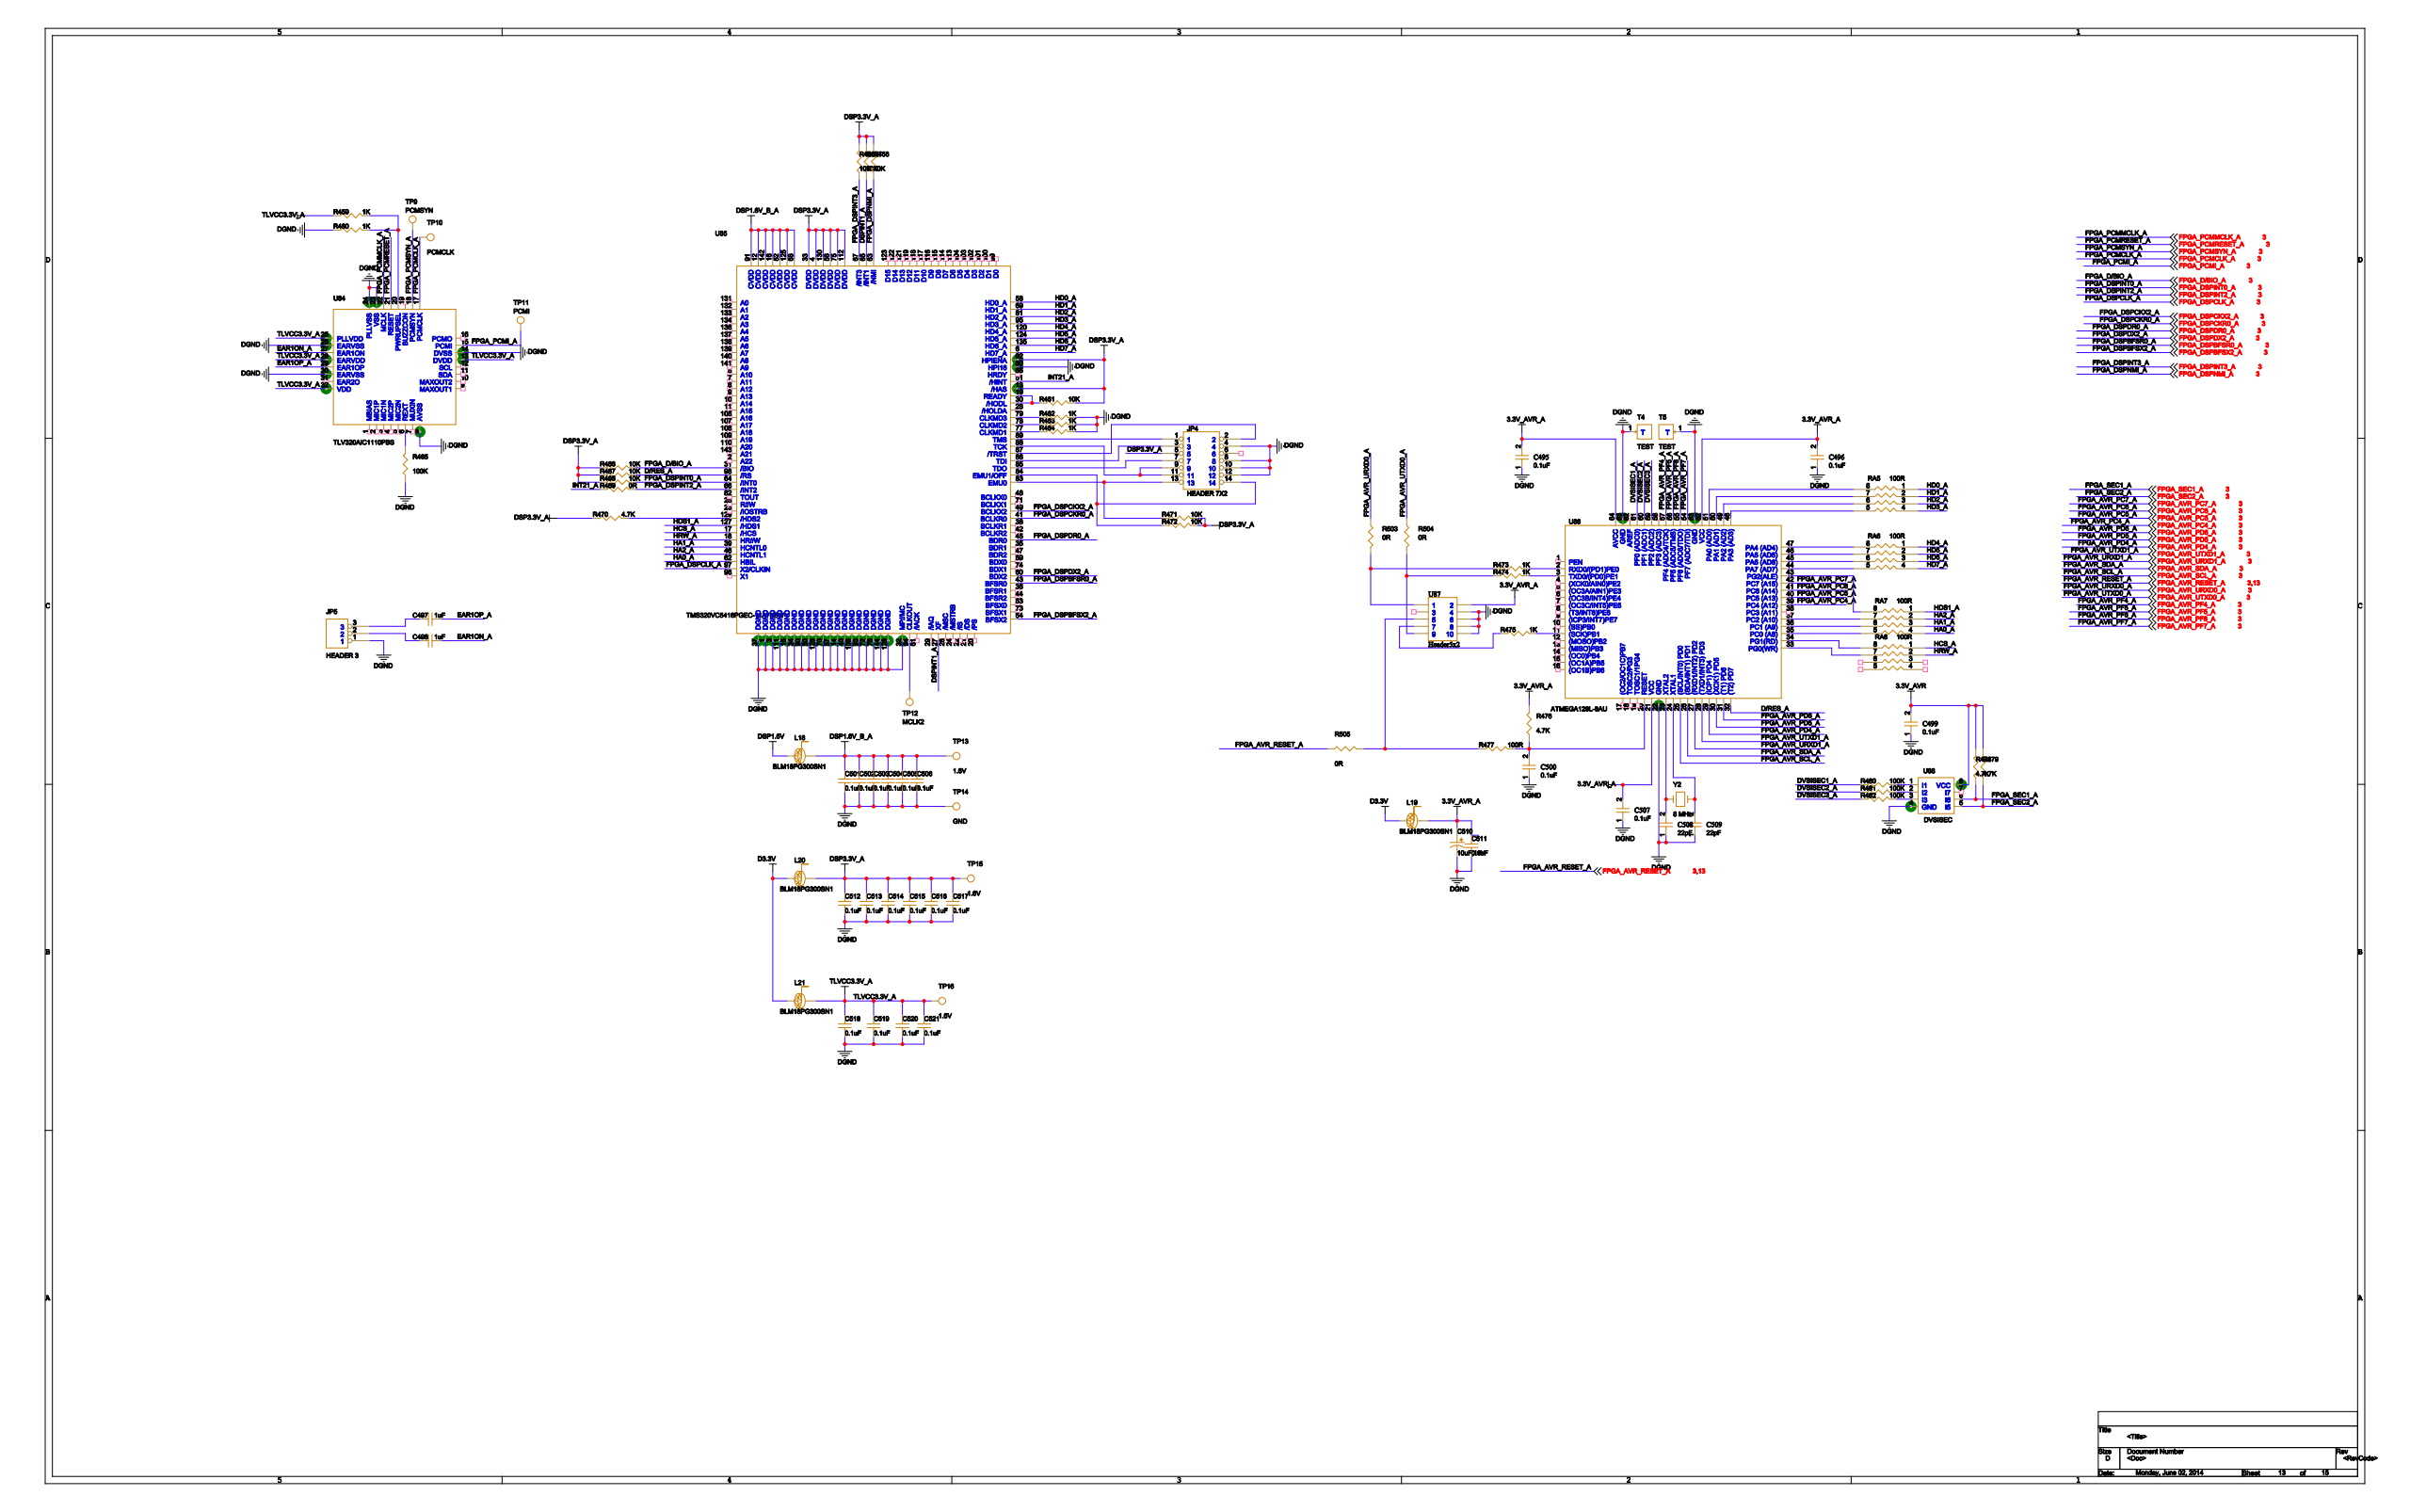Circuit board | Cadence Allegro | 669 parts | 806 nets | one sheet of the schematic
Parts on this sheet (reference | value | footprint):
C495 | 0.1uF | C0402
C496 | 0.1uF | C0402
C497 | 1uF | C0603
C498 | 1uF | C0603
C499 | 0.1uF | C0402
C500 | 0.1uF | C0402
C501 | 0.1uF | C0402
C502 | 0.1uF | C0402
C503 | 0.1uF | C0402
C504 | 0.1uF | C0402
C505 | 0.1uF | C0402
C506 | 0.1uF | C0402
C507 | 0.1uF | C0402
C508 | 22pF | C0402
C509 | 22pF | C0402
C510 | 10uF,16V | CP3216
C511 | 0.1uF | C0402
C512 | 0.1uF | C0402
C513 | 0.1uF | C0402
C514 | 0.1uF | C0402
C515 | 0.1uF | C0402
C516 | 0.1uF | C0402
C517 | 0.1uF | C0402
C518 | 0.1uF | C0402
C519 | 0.1uF | C0402
C520 | 0.1uF | C0402
C521 | 0.1uF | C0402
JP4 | HEADER 7X2 | SIP14_254
JP5 | HEADER 3 | ZIP3
L18 | BLM18PG300SN1 | F0603
L19 | BLM18PG300SN1 | F0603
L20 | BLM18PG300SN1 | F0603
L21 | BLM18PG300SN1 | F0603
R456 | 10K | R0603
R457 | 10K | R0603
R458 | 10K | R0603
R459 | 1K | R0603
R460 | 1K | R0603
R461 | 10K | R0603
R462 | 1K | R0603
R463 | 1K | R0603
R464 | 1K | R0603
R465 | 100K | R0603
R466 | 10K | R0603
R467 | 10K | R0603
R468 | 10K | R0603
R469 | 0R | R0603
R470 | 4.7K | R0603
R471 | 10K | R0603
R472 | 10K | R0603
R473 | 1K | R0603
R474 | 1K | R0603
R475 | 1K | R0603
R476 | 4.7K | R0603
R477 | 100R | R0603
R478 | 4.7K | R0603
R479 | 4.7K | R0603
R480 | 100K | R0603
R481 | 100K | R0603
R482 | 100K | R0603
R503 | 0R | R0603
R504 | 0R | R0603
R505 | 0R | R0603
RA5 | 100R | 8P4R0603
RA6 | 100R | 8P4R0603
RA7 | 100R | 8P4R0603
RA8 | 100R | 8P4R0603
T4 | TEST | SMD1
T5 | TEST | SMD1
TP9 | PCMSYN | SIP1
TP10 | PCMCLK | SIP1
TP11 | PCMI | SIP1
TP12 | MCLK2 | SIP1
TP13 | 1.6V | SIP1
TP14 | GND | SIP1
TP15 | 1.6V | SIP1
TP16 | 1.6V | SIP1
U84 | TLV320AIC1110PBS | QFP32_0P5M_7X7M
U85 | TMS320VC5416PGEC-11A7K8W | QFP144_0P5M_22X22M
U86 | ATMEGA128L-8AU | QFP64_0P8M_16X16M
U87 | Header5x2 | ZIP10
U88 | DVSISEC | SOP8_1P27M_6X5M
Nets of these parts (net: part-pin ...):
DGND: C495-1 C496-1 C499-1 C500-1 C501-2 C502-2 C503-2 C504-2 C505-2 C506-2 C507-1 C508-1 C509-1 C510-2 C511-2 C512-2 C513-2 C514-2 C515-2 C516-2 C517-2 C518-2 C519-2 C520-2 C521-2 JP4-4 JP4-8 JP4-10 JP4-12 JP5-1 R460-1 R462-2 R463-2 R464-2 R465-1 T4-1 T5-1 TP14-1 U84-8 U84-14 U84-23 U84-24 U84-26 U84-30 U87-4 U87-6 U87-8 U87-10 U88-4 U85-1 U85-3 U85-14 U85-15 U85-32 U85-34 U85-37 U85-40 U85-50 U85-57 U85-70 U85-72 U85-76 U85-80 U85-90 U85-93 U85-106 U85-111 U85-126 U85-128 U85-144 U86-22 U86-53 U86-63
3.3V_AVR: C499-2 R478-2 R479-2 U88-8
N60953702: R480-2 U88-1
N60953704: R481-2 U88-2
N60953706: R482-2 U88-3
FPGA_SEC2_A: R479-1 U88-5
FPGA_SEC1_A: R478-1 U88-6
FPGA_AVR_PC7_A: U86-42
FPGA_AVR_PC6_A: U86-41
FPGA_PCMI_A: TP11-1 U84-15
FPGA_PCMCLK_A: TP10-1 U84-17
FPGA_AVR_URXD1_A: U86-27
FPGA_AVR_PC5_A: U86-40
FPGA_AVR_PD5_A: U86-30
FPGA_AVR_PD6_A: U86-31
FPGA_AVR_PC4_A: U86-39
FPGA_PCMRESET_A: U84-21
FPGA_PCMSYN_A: TP9-1 U84-18
FPGA_AVR_UTXD0_A: R504-1
FPGA_AVR_URXD0_A: R503-1
FPGA_AVR_SDA_A: U86-26
FPGA_AVR_SCL_A: U86-25
FPGA_AVR_UTXD1_A: U86-28
FPGA_AVR_PD4_A: U86-29
FPGA_DSPCKX2_A: U85-49
FPGA_DSPCKR0_A: U85-41
FPGA_DSPDR0_A: U85-45
FPGA_DSPINT3_A: R456-1 U85-67
FPGA_AVR_RESET_A: R505-1
FPGA_AVR_PF6_A: U86-55
FPGA_PCMMCLK_A: U84-22
FPGA_DSPNMI_A: R458-1 U85-63
FPGA_DSPDX2_A: U85-60
FPGA_DSPINT2_A: R469-2 U85-66
FPGA_DSPINT0_A: R468-2 U85-64
FPGA_AVR_PF7_A: U86-54
FPGA_AVR_PF4_A: U86-57
FPGA_AVR_PF5_A: U86-56
FPGA_D/BIO_A: R466-2 U85-31
FPGA_DSPBFSR0_A: U85-43
FPGA_DSPBFSX2_A: U85-54
FPGA_DSPCLK_A: U85-97
TLVCC3.3V_A: C518-1 C519-1 C520-1 C521-1 L21-2 R459-1 TP16-1 U84-13 U84-25 U84-28 U84-32
EAR1ON_A: C498-2 U84-27
EAR1OP_A: C497-2 U84-29
N16284419: R459-2 R460-2 U84-20
N16284265: R465-2 U84-6
N60953958: R475-2 U86-11
D/RES_A: R467-2 U85-98 U86-32
3.3V_AVR_A: C495-2 C496-2 C507-2 C510-1 C511-1 L19-2 R476-2 U87-2 U86-21 U86-52 U86-64
N60953825: RA5-8 U86-51
N60953829: RA5-7 U86-50
N60953817: RA5-6 U86-49
N60953821: RA5-5 U86-48
N60953833: RA6-8 U86-47
N60953835: RA6-7 U86-46
N60953837: RA6-6 U86-45
N60953839: RA6-5 U86-44
N60953845: RA7-5 U86-35
N60953855: RA7-6 U86-36
N60953857: RA7-7 U86-37
DVSISEC1_A: R480-1 U86-61
DVSISEC2_A: R481-1 U86-60
DVSISEC3_A: R482-1 U86-59
N60953843: RA8-7 U86-33
N60953841: RA8-8 U86-34
N60953859: RA7-8 U86-43
N60953989: C500-2 R476-1 R477-2 U86-20
N60953932: R473-2 U86-2
N60953934: R474-2 U86-3
N60953700: C509-2 U86-24
N60953698: C508-2 U86-23
N61571160: JP4-1 U85-89
N16285005: JP4-9 JP4-11 U85-88
N16285187: JP4-13 R471-1 U85-83
N16285167: JP4-14 R472-1 U85-84
N16285017: JP4-2 U85-87
N16285045: JP4-3 U85-86
DSP3.3V_A: C512-1 C513-1 C514-1 C515-1 C516-1 C517-1 JP4-5 L20-2 R456-2 R457-2 R458-2 R461-2 R466-1 R467-1 R468-1 R470-1 R471-2 R472-2 TP15-1 U85-4 U85-13 U85-33 U85-56 U85-75 U85-92 U85-112 U85-130
N16285061: JP4-7 U85-85
N60953940: R473-1 R503-2 U87-1
N60953943: R474-1 R504-2 U87-9
N60953982: R477-1 R505-2 U87-5
INT21_A: R469-1 U85-51
D3.3V: L19-1 L20-1 L21-1
HD0_A: RA5-1 U85-58
HD1_A: RA5-2 U85-69
HD2_A: RA5-3 U85-81
HD3_A: RA5-4 U85-95
HD4_A: RA6-1 U85-120
HD5_A: RA6-2 U85-124
HD6_A: RA6-3 U85-135
HD7_A: RA6-4 U85-6
HDS1_A: RA7-1 U85-127
HA2_A: RA7-2 U85-46
HA1_A: RA7-3 U85-39
HA0_A: RA7-4 U85-62
HCS_A: RA8-1 U85-17
HRW_A: RA8-2 U85-18
N16288187: R470-2 U85-129
N16284861: R461-1 U85-19 U85-30
DSPINT1_A: R457-1 U85-27 U85-65
N16284933: R464-1 U85-77
N16284929: R463-1 U85-78
N16284925: R462-1 U85-79
N16285409: TP12-1 U85-94
DSP1.6V_B_A: C501-1 C502-1 C503-1 C504-1 C505-1 C506-1 L18-2 TP13-1 U85-12 U85-16 U85-52 U85-68 U85-91 U85-125 U85-142
N16285385: C497-1 JP5-3
N16285373: C498-1 JP5-2
N60953954: R475-1 U87-7
DSP1.6V: L18-1